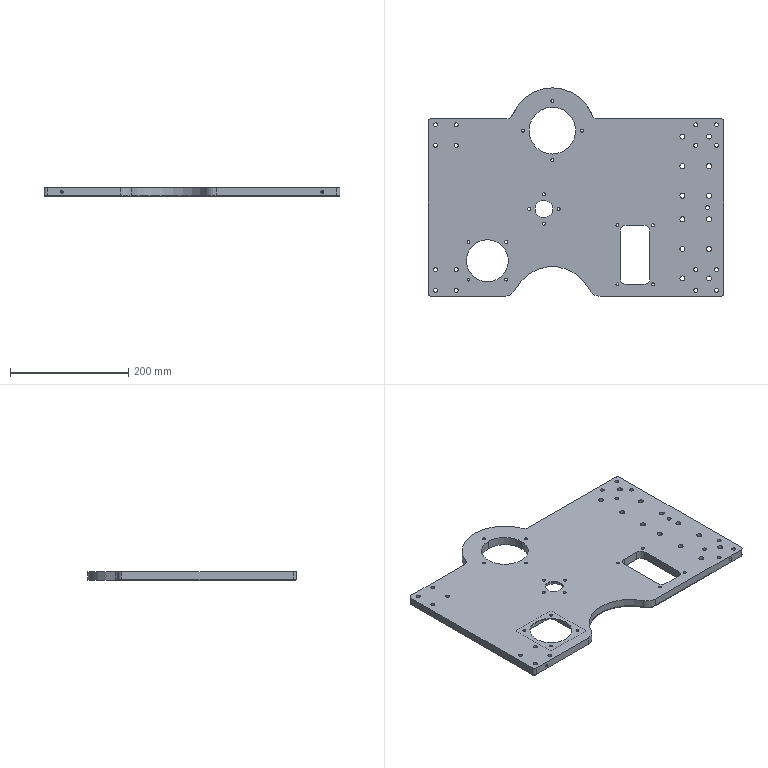Part | 1 solid | 222 faces | volume 1941291 mm3 | cylinder 168 | plane 37 | cone 8 | torus 7 | spline 2 | commonest cylinder face diameters 5 x40 6.6 x32 11 x32 8.5 x24 4 x14 20 x6